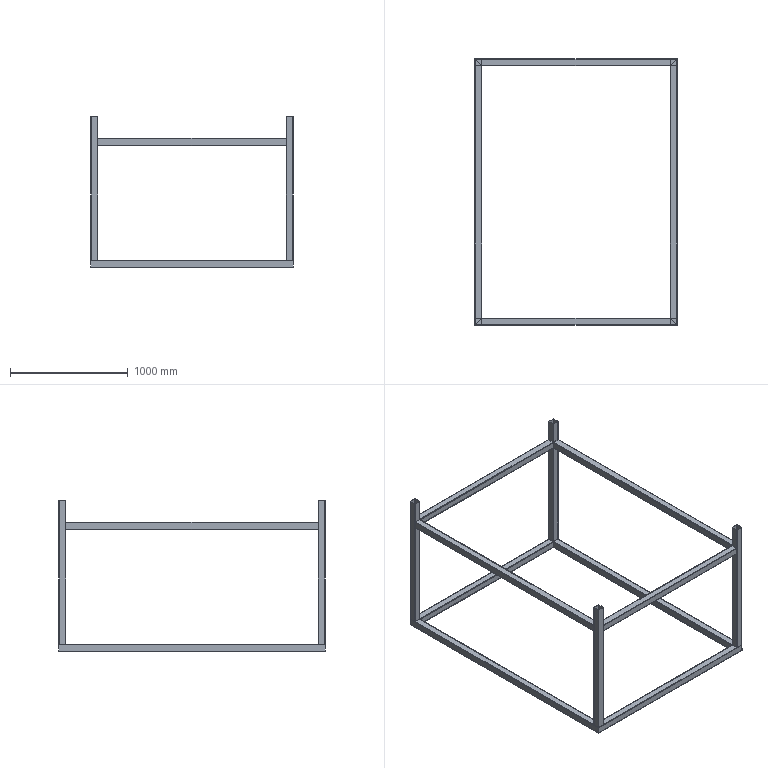Part | STEP file | Part 38_Default<Machined> | 12 solids | 216 faces | box 1720 x 2260 x 1280 mm | volume 9110278 mm3 | plane 120 | cylinder 96 | commonest cylinder face diameters 4 x48 8 x48